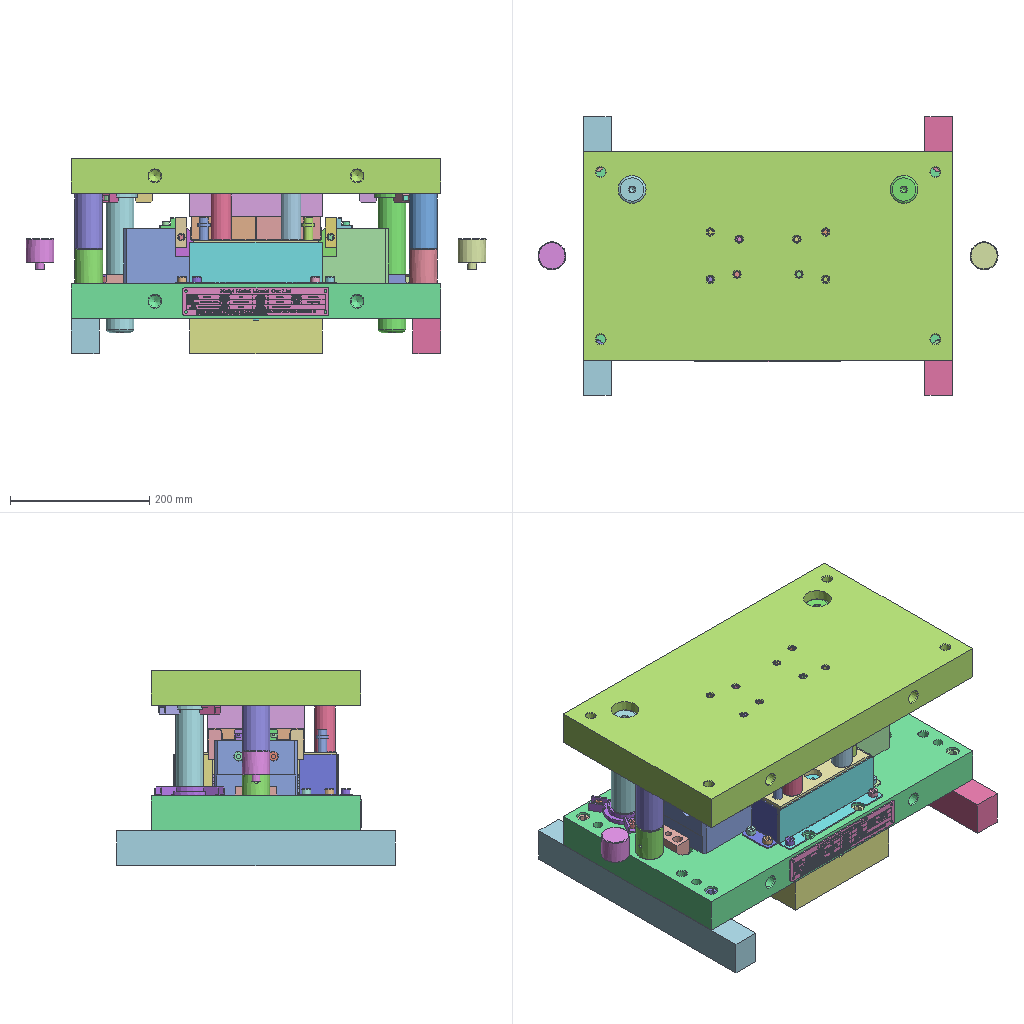Assembly | STEP file | 269 different items | 269 placed | box 660 x 400 x 280 mm
Parts list (item | name | quantity | parent item | size | volume):
1 | gslz 2016.10.28-6_id1002_x_t | x1 | in gslz 2016.10.28-6_x_t | 28.004 x 12 x 21.002 mm | 4222 mm3
2 | gslz 2016.10.28-6_id1006_x_t | x1 | in gslz 2016.10.28-6_x_t | 16 x 20 x 42.992 mm | 9660 mm3
3 | gslz 2016.10.28-6_id1010_x_t | x1 | in gslz 2016.10.28-6_x_t | 190 x 22 x 60 mm | 28864 mm3
4 | gslz 2016.10.28-6_id1014_x_t | x1 | in gslz 2016.10.28-6_x_t | - | 16189 mm3
5 | gslz 2016.10.28-6_id1018_x_t | x1 | in gslz 2016.10.28-6_x_t | 23 x 53 x 60 mm | 8271 mm3
6 | gslz 2016.10.28-6_id1022_x_t | x1 | in gslz 2016.10.28-6_x_t | 23 x 53 x 60 mm | 8271 mm3
7 | gslz 2016.10.28-6_id1026_x_t | x1 | in gslz 2016.10.28-6_x_t | 30 x 30 x 67.992 mm | 42323 mm3
8 | gslz 2016.10.28-6_id102_x_t | x1 | in gslz 2016.10.28-6_x_t | 18 x 18 x 67 mm | 8561 mm3
9 | gslz 2016.10.28-6_id1030_x_t | x1 | in gslz 2016.10.28-6_x_t | 30 x 30 x 67.992 mm | 42323 mm3
10 | gslz 2016.10.28-6_id1034_x_t | x1 | in gslz 2016.10.28-6_x_t | 25 x 110 x 40 mm | 96354 mm3
11 | gslz 2016.10.28-6_id1038_x_t | x1 | in gslz 2016.10.28-6_x_t | 190 x 300 x 50 mm | 2589810 mm3
12 | gslz 2016.10.28-6_id1042_x_t | x1 | in gslz 2016.10.28-6_x_t | 30 x 30 x 67.992 mm | 42323 mm3
13 | gslz 2016.10.28-6_id1046_x_t | x1 | in gslz 2016.10.28-6_x_t | 30 x 30 x 67.992 mm | 42323 mm3
14 | gslz 2016.10.28-6_id1050_x_t | x1 | in gslz 2016.10.28-6_x_t | 9.497 x 9.497 x 27.381 mm | 1219 mm3
15 | gslz 2016.10.28-6_id1054_x_t | x1 | in gslz 2016.10.28-6_x_t | 9.497 x 9.497 x 27.383 mm | 1219 mm3
16 | gslz 2016.10.28-6_id1058_x_t | x1 | in gslz 2016.10.28-6_x_t | 9.497 x 9.497 x 27.391 mm | 1219 mm3
17 | gslz 2016.10.28-6_id1062_x_t | x1 | in gslz 2016.10.28-6_x_t | 30 x 30 x 30 mm | 18212 mm3
18 | gslz 2016.10.28-6_id1066_x_t | x1 | in gslz 2016.10.28-6_x_t | 9.497 x 9.497 x 27.391 mm | 1219 mm3
19 | gslz 2016.10.28-6_id106_x_t | x1 | in gslz 2016.10.28-6_x_t | 18 x 18 x 67 mm | 8561 mm3
20 | gslz 2016.10.28-6_id1070_x_t | x1 | in gslz 2016.10.28-6_x_t | 530 x 300 x 50 mm | 7668211 mm3
21 | gslz 2016.10.28-6_id1074_x_t | x1 | in gslz 2016.10.28-6_x_t | 100 x 120 x 79 mm | 734438 mm3
22 | gslz 2016.10.28-6_id1078_x_t | x1 | in gslz 2016.10.28-6_x_t | 92 x 138 x 33.5 mm | 325352 mm3
23 | gslz 2016.10.28-6_id10_x_t | x1 | in gslz 2016.10.28-6_x_t | 25 x 60 x 25 mm | 30776 mm3
24 | gslz 2016.10.28-6_id110_x_t | x1 | in gslz 2016.10.28-6_x_t | 18 x 18 x 67 mm | 8561 mm3
25 | gslz 2016.10.28-6_id114_x_t | x1 | in gslz 2016.10.28-6_x_t | 18 x 18 x 67 mm | 8561 mm3
26 | gslz 2016.10.28-6_id118_x_t | x1 | in gslz 2016.10.28-6_x_t | 18 x 18 x 67 mm | 8561 mm3
27 | gslz 2016.10.28-6_id122_x_t | x1 | in gslz 2016.10.28-6_x_t | 13 x 13 x 23 mm | 1651 mm3
28 | gslz 2016.10.28-6_id126_x_t | x1 | in gslz 2016.10.28-6_x_t | 13 x 13 x 23 mm | 1651 mm3
29 | gslz 2016.10.28-6_id130_x_t | x1 | in gslz 2016.10.28-6_x_t | 13 x 13 x 23 mm | 1651 mm3
30 | gslz 2016.10.28-6_id134_x_t | x1 | in gslz 2016.10.28-6_x_t | 13 x 13 x 23 mm | 1651 mm3
31 | gslz 2016.10.28-6_id138_x_t | x1 | in gslz 2016.10.28-6_x_t | 13 x 13 x 23 mm | 1651 mm3
32 | gslz 2016.10.28-6_id142_x_t | x1 | in gslz 2016.10.28-6_x_t | 13 x 13 x 23 mm | 1651 mm3
33 | gslz 2016.10.28-6_id146_x_t | x1 | in gslz 2016.10.28-6_x_t | 13 x 13 x 23 mm | 1651 mm3
34 | gslz 2016.10.28-6_id14_x_t | x1 | in gslz 2016.10.28-6_x_t | 530 x 300 x 50 mm | 6912423 mm3
35 | gslz 2016.10.28-6_id150_x_t | x1 | in gslz 2016.10.28-6_x_t | 13 x 13 x 23 mm | 1651 mm3
36 | gslz 2016.10.28-6_id154_x_t | x1 | in gslz 2016.10.28-6_x_t | 13 x 13 x 23 mm | 1651 mm3
37 | gslz 2016.10.28-6_id158_x_t | x1 | in gslz 2016.10.28-6_x_t | 13 x 13 x 23 mm | 1651 mm3
38 | gslz 2016.10.28-6_id162_x_t | x1 | in gslz 2016.10.28-6_x_t | 13 x 13 x 23 mm | 1651 mm3
39 | gslz 2016.10.28-6_id166_x_t | x1 | in gslz 2016.10.28-6_x_t | 13 x 13 x 23 mm | 1651 mm3
40 | gslz 2016.10.28-6_id170_x_t | x1 | in gslz 2016.10.28-6_x_t | 40 x 40 x 50 mm | 56993 mm3
41 | gslz 2016.10.28-6_id174_x_t | x1 | in gslz 2016.10.28-6_x_t | 40 x 40 x 80 mm | 91705 mm3
42 | gslz 2016.10.28-6_id178_x_t | x1 | in gslz 2016.10.28-6_x_t | 13 x 13 x 52 mm | 3108 mm3
43 | gslz 2016.10.28-6_id182_x_t | x1 | in gslz 2016.10.28-6_x_t | 13 x 13 x 82 mm | 4616 mm3
44 | gslz 2016.10.28-6_id186_x_t | x1 | in gslz 2016.10.28-6_x_t | 40 x 40 x 45 mm | 44861 mm3
45 | gslz 2016.10.28-6_id18_x_t | x1 | in gslz 2016.10.28-6_x_t | 20 x 40 x 20 mm | 14270 mm3
46 | gslz 2016.10.28-6_id190_x_t | x1 | in gslz 2016.10.28-6_x_t | 40 x 40 x 45 mm | 44861 mm3
47 | gslz 2016.10.28-6_id194_x_t | x1 | in gslz 2016.10.28-6_x_t | 40 x 40 x 80 mm | 91705 mm3
48 | gslz 2016.10.28-6_id198_x_t | x1 | in gslz 2016.10.28-6_x_t | 40 x 40 x 50 mm | 56993 mm3
49 | gslz 2016.10.28-6_id202_x_t | x1 | in gslz 2016.10.28-6_x_t | 13 x 13 x 52 mm | 3108 mm3
50 | gslz 2016.10.28-6_id206_x_t | x1 | in gslz 2016.10.28-6_x_t | 13 x 13 x 82 mm | 4616 mm3
51 | gslz 2016.10.28-6_id210_x_t | x1 | in gslz 2016.10.28-6_x_t | 13 x 13 x 77 mm | 4365 mm3
52 | gslz 2016.10.28-6_id214_x_t | x1 | in gslz 2016.10.28-6_x_t | 13 x 13 x 77 mm | 4365 mm3
53 | gslz 2016.10.28-6_id218_x_t | x1 | in gslz 2016.10.28-6_x_t | 13 x 13 x 77 mm | 4365 mm3
54 | gslz 2016.10.28-6_id222_x_t | x1 | in gslz 2016.10.28-6_x_t | 13 x 13 x 77 mm | 4365 mm3
55 | gslz 2016.10.28-6_id226_x_t | x1 | in gslz 2016.10.28-6_x_t | 13 x 13 x 48 mm | 2907 mm3
56 | gslz 2016.10.28-6_id22_x_t | x1 | in gslz 2016.10.28-6_x_t | 180 x 230 x 32 mm | 1103435 mm3
57 | gslz 2016.10.28-6_id230_x_t | x1 | in gslz 2016.10.28-6_x_t | 13 x 13 x 48 mm | 2907 mm3
58 | gslz 2016.10.28-6_id234_x_t | x1 | in gslz 2016.10.28-6_x_t | 10 x 10 x 27 mm | 972.376 mm3
59 | gslz 2016.10.28-6_id238_x_t | x1 | in gslz 2016.10.28-6_x_t | 40 x 16 x 16 mm | 8856 mm3
60 | gslz 2016.10.28-6_id242_x_t | x1 | in gslz 2016.10.28-6_x_t | 10 x 10 x 27 mm | 972.376 mm3
61 | gslz 2016.10.28-6_id246_x_t | x1 | in gslz 2016.10.28-6_x_t | 16 x 40 x 16 mm | 8856 mm3
62 | gslz 2016.10.28-6_id250_x_t | x1 | in gslz 2016.10.28-6_x_t | 10 x 10 x 27 mm | 972.376 mm3
63 | gslz 2016.10.28-6_id254_x_t | x1 | in gslz 2016.10.28-6_x_t | 16 x 40 x 16 mm | 8856 mm3
64 | gslz 2016.10.28-6_id258_x_t | x1 | in gslz 2016.10.28-6_x_t | 10 x 10 x 26 mm | 944.102 mm3
65 | gslz 2016.10.28-6_id262_x_t | x1 | in gslz 2016.10.28-6_x_t | 30 x 16 x 16 mm | 6296 mm3
66 | gslz 2016.10.28-6_id266_x_t | x1 | in gslz 2016.10.28-6_x_t | 10 x 10 x 27 mm | 972.376 mm3
67 | gslz 2016.10.28-6_id26_x_t | x1 | in gslz 2016.10.28-6_x_t | 43 x 62 x 89 mm | 180403 mm3
68 | gslz 2016.10.28-6_id270_x_t | x1 | in gslz 2016.10.28-6_x_t | 16 x 40 x 16 mm | 8856 mm3
69 | gslz 2016.10.28-6_id274_x_t | x1 | in gslz 2016.10.28-6_x_t | 10 x 10 x 27 mm | 972.376 mm3
70 | gslz 2016.10.28-6_id278_x_t | x1 | in gslz 2016.10.28-6_x_t | 16 x 40 x 16 mm | 8856 mm3
71 | gslz 2016.10.28-6_id282_x_t | x1 | in gslz 2016.10.28-6_x_t | 10 x 10 x 26 mm | 944.102 mm3
72 | gslz 2016.10.28-6_id286_x_t | x1 | in gslz 2016.10.28-6_x_t | 30 x 16 x 16 mm | 6296 mm3
73 | gslz 2016.10.28-6_id290_x_t | x1 | in gslz 2016.10.28-6_x_t | 16 x 16 x 85 mm | 7560 mm3
74 | gslz 2016.10.28-6_id294_x_t | x1 | in gslz 2016.10.28-6_x_t | 16 x 16 x 85 mm | 7560 mm3
75 | gslz 2016.10.28-6_id298_x_t | x1 | in gslz 2016.10.28-6_x_t | 16 x 16 x 85 mm | 7560 mm3
76 | gslz 2016.10.28-6_id302_x_t | x1 | in gslz 2016.10.28-6_x_t | 16 x 16 x 85 mm | 7560 mm3
77 | gslz 2016.10.28-6_id306_x_t | x1 | in gslz 2016.10.28-6_x_t | 16 x 16 x 85 mm | 7560 mm3
78 | gslz 2016.10.28-6_id30_x_t | x1 | in gslz 2016.10.28-6_x_t | 43 x 62 x 89 mm | 180403 mm3
79 | gslz 2016.10.28-6_id310_x_t | x1 | in gslz 2016.10.28-6_x_t | 16 x 16 x 85 mm | 7560 mm3
80 | gslz 2016.10.28-6_id314_x_t | x1 | in gslz 2016.10.28-6_x_t | 16 x 16 x 85 mm | 7560 mm3
81 | gslz 2016.10.28-6_id318_x_t | x1 | in gslz 2016.10.28-6_x_t | 16 x 16 x 85 mm | 7560 mm3
82 | gslz 2016.10.28-6_id322_x_t | x1 | in gslz 2016.10.28-6_x_t | 190 x 138 x 33 mm | 763181 mm3
83 | gslz 2016.10.28-6_id326_x_t | x1 | in gslz 2016.10.28-6_x_t | 12 x 12 x 12 mm | 1092 mm3
84 | gslz 2016.10.28-6_id330_x_t | x1 | in gslz 2016.10.28-6_x_t | 9.997 x 9.994 x 45 mm | 331.132 mm3
85 | gslz 2016.10.28-6_id334_x_t | x1 | in gslz 2016.10.28-6_x_t | 10 x 10 x 48 mm | 2492 mm3
86 | gslz 2016.10.28-6_id338_x_t | x1 | in gslz 2016.10.28-6_x_t | 9.997 x 9.994 x 45 mm | 331.132 mm3
87 | gslz 2016.10.28-6_id342_x_t | x1 | in gslz 2016.10.28-6_x_t | 12 x 12 x 12 mm | 1092 mm3
88 | gslz 2016.10.28-6_id346_x_t | x1 | in gslz 2016.10.28-6_x_t | 10 x 10 x 48 mm | 2492 mm3
89 | gslz 2016.10.28-6_id34_x_t | x1 | in gslz 2016.10.28-6_x_t | 43 x 62 x 89 mm | 180411 mm3
90 | gslz 2016.10.28-6_id350_x_t | x1 | in gslz 2016.10.28-6_x_t | 9.997 x 9.994 x 45 mm | 331.132 mm3
91 | gslz 2016.10.28-6_id354_x_t | x1 | in gslz 2016.10.28-6_x_t | 12 x 12 x 12 mm | 1092 mm3
92 | gslz 2016.10.28-6_id358_x_t | x1 | in gslz 2016.10.28-6_x_t | 10 x 10 x 48 mm | 2492 mm3
93 | gslz 2016.10.28-6_id362_x_t | x1 | in gslz 2016.10.28-6_x_t | 9.997 x 9.994 x 45 mm | 331.132 mm3
94 | gslz 2016.10.28-6_id366_x_t | x1 | in gslz 2016.10.28-6_x_t | 12 x 12 x 12 mm | 1092 mm3
95 | gslz 2016.10.28-6_id370_x_t | x1 | in gslz 2016.10.28-6_x_t | 10 x 10 x 48 mm | 2492 mm3
96 | gslz 2016.10.28-6_id374_x_t | x1 | in gslz 2016.10.28-6_x_t | 9.997 x 9.994 x 45 mm | 330.149 mm3
97 | gslz 2016.10.28-6_id378_x_t | x1 | in gslz 2016.10.28-6_x_t | 12 x 12 x 12 mm | 1092 mm3
98 | gslz 2016.10.28-6_id382_x_t | x1 | in gslz 2016.10.28-6_x_t | 10 x 10 x 48 mm | 2492 mm3
99 | gslz 2016.10.28-6_id386_x_t | x1 | in gslz 2016.10.28-6_x_t | 9.997 x 9.994 x 45 mm | 330.149 mm3
100 | gslz 2016.10.28-6_id38_x_t | x1 | in gslz 2016.10.28-6_x_t | 82.449 x 96 x 19.004 mm | 9470 mm3
101 | gslz 2016.10.28-6_id390_x_t | x1 | in gslz 2016.10.28-6_x_t | 12 x 12 x 12 mm | 1092 mm3
102 | gslz 2016.10.28-6_id394_x_t | x1 | in gslz 2016.10.28-6_x_t | 10 x 10 x 48 mm | 2492 mm3
103 | gslz 2016.10.28-6_id398_x_t | x1 | in gslz 2016.10.28-6_x_t | 12 x 12 x 12 mm | 1092 mm3
104 | gslz 2016.10.28-6_id402_x_t | x1 | in gslz 2016.10.28-6_x_t | 9.997 x 9.994 x 45 mm | 330.149 mm3
105 | gslz 2016.10.28-6_id406_x_t | x1 | in gslz 2016.10.28-6_x_t | 10 x 10 x 48 mm | 2492 mm3
106 | gslz 2016.10.28-6_id410_x_t | x1 | in gslz 2016.10.28-6_x_t | 12 x 12 x 12 mm | 1092 mm3
107 | gslz 2016.10.28-6_id414_x_t | x1 | in gslz 2016.10.28-6_x_t | 10 x 10 x 48 mm | 2492 mm3
108 | gslz 2016.10.28-6_id418_x_t | x1 | in gslz 2016.10.28-6_x_t | 9.997 x 9.994 x 45 mm | 330.149 mm3
109 | gslz 2016.10.28-6_id422_x_t | x1 | in gslz 2016.10.28-6_x_t | 10 x 10 x 26 mm | 944.102 mm3
110 | gslz 2016.10.28-6_id426_x_t | x1 | in gslz 2016.10.28-6_x_t | 10 x 10 x 26 mm | 944.102 mm3
111 | gslz 2016.10.28-6_id42_x_t | x1 | in gslz 2016.10.28-6_x_t | 92 x 138 x 33.5 mm | 323745 mm3
112 | gslz 2016.10.28-6_id430_x_t | x1 | in gslz 2016.10.28-6_x_t | 10 x 10 x 26 mm | 944.102 mm3
113 | gslz 2016.10.28-6_id434_x_t | x1 | in gslz 2016.10.28-6_x_t | 56.6 x 32.6 x 114 mm | 58332 mm3
114 | gslz 2016.10.28-6_id438_x_t | x1 | in gslz 2016.10.28-6_x_t | 10 x 10 x 26 mm | 944.102 mm3
115 | gslz 2016.10.28-6_id442_x_t | x1 | in gslz 2016.10.28-6_x_t | 64 x 40 x 40 mm | 16525 mm3
116 | gslz 2016.10.28-6_id446_x_t | x1 | in gslz 2016.10.28-6_x_t | 10 x 10 x 26 mm | 944.102 mm3
117 | gslz 2016.10.28-6_id450_x_t | x1 | in gslz 2016.10.28-6_x_t | 64 x 40 x 40 mm | 16525 mm3
118 | gslz 2016.10.28-6_id454_x_t | x1 | in gslz 2016.10.28-6_x_t | 10 x 10 x 26 mm | 944.102 mm3
119 | gslz 2016.10.28-6_id458_x_t | x1 | in gslz 2016.10.28-6_x_t | 10 x 10 x 26 mm | 944.102 mm3
120 | gslz 2016.10.28-6_id462_x_t | x1 | in gslz 2016.10.28-6_x_t | 10 x 10 x 26 mm | 944.102 mm3
121 | gslz 2016.10.28-6_id466_x_t | x1 | in gslz 2016.10.28-6_x_t | 56.6 x 32.6 x 114 mm | 58331 mm3
122 | gslz 2016.10.28-6_id46_x_t | x1 | in gslz 2016.10.28-6_x_t | 82.449 x 96 x 19.004 mm | 9463 mm3
123 | gslz 2016.10.28-6_id470_x_t | x1 | in gslz 2016.10.28-6_x_t | 12 x 12 x 12 mm | 1092 mm3
124 | gslz 2016.10.28-6_id474_x_t | x1 | in gslz 2016.10.28-6_x_t | 12 x 12 x 12 mm | 1092 mm3
125 | gslz 2016.10.28-6_id478_x_t | x1 | in gslz 2016.10.28-6_x_t | 12 x 12 x 12 mm | 1092 mm3
126 | gslz 2016.10.28-6_id482_x_t | x1 | in gslz 2016.10.28-6_x_t | 12 x 12 x 12 mm | 1092 mm3
127 | gslz 2016.10.28-6_id486_x_t | x1 | in gslz 2016.10.28-6_x_t | 18 x 18 x 110 mm | 13813 mm3
128 | gslz 2016.10.28-6_id490_x_t | x1 | in gslz 2016.10.28-6_x_t | 18 x 18 x 110 mm | 13813 mm3
129 | gslz 2016.10.28-6_id494_x_t | x1 | in gslz 2016.10.28-6_x_t | 18 x 18 x 110 mm | 13813 mm3
130 | gslz 2016.10.28-6_id498_x_t | x1 | in gslz 2016.10.28-6_x_t | 18 x 18 x 110 mm | 13813 mm3
131 | gslz 2016.10.28-6_id502_x_t | x1 | in gslz 2016.10.28-6_x_t | 6 x 6 x 13 mm | 209.85 mm3
132 | gslz 2016.10.28-6_id506_x_t | x1 | in gslz 2016.10.28-6_x_t | 8 x 8 x 8 mm | 323.66 mm3
133 | gslz 2016.10.28-6_id50_x_t | x1 | in gslz 2016.10.28-6_x_t | 40.005 x 40.005 x 103 mm | 60665 mm3
134 | gslz 2016.10.28-6_id510_x_t | x1 | in gslz 2016.10.28-6_x_t | 5.996 x 5.994 x 11 mm | 66.438 mm3
135 | gslz 2016.10.28-6_id514_x_t | x1 | in gslz 2016.10.28-6_x_t | 6 x 6 x 13 mm | 209.85 mm3
136 | gslz 2016.10.28-6_id518_x_t | x1 | in gslz 2016.10.28-6_x_t | 8 x 8 x 8 mm | 323.66 mm3
137 | gslz 2016.10.28-6_id522_x_t | x1 | in gslz 2016.10.28-6_x_t | 5.996 x 5.994 x 11 mm | 66.438 mm3
138 | gslz 2016.10.28-6_id526_x_t | x1 | in gslz 2016.10.28-6_x_t | 6 x 6 x 13 mm | 209.85 mm3
139 | gslz 2016.10.28-6_id530_x_t | x1 | in gslz 2016.10.28-6_x_t | 8 x 8 x 8 mm | 323.66 mm3
140 | gslz 2016.10.28-6_id534_x_t | x1 | in gslz 2016.10.28-6_x_t | 5.996 x 5.994 x 11 mm | 66.438 mm3
141 | gslz 2016.10.28-6_id538_x_t | x1 | in gslz 2016.10.28-6_x_t | 6 x 6 x 13 mm | 209.85 mm3
142 | gslz 2016.10.28-6_id542_x_t | x1 | in gslz 2016.10.28-6_x_t | 8 x 8 x 8 mm | 323.66 mm3
143 | gslz 2016.10.28-6_id546_x_t | x1 | in gslz 2016.10.28-6_x_t | 5.996 x 5.994 x 11 mm | 66.438 mm3
144 | gslz 2016.10.28-6_id54_x_t | x1 | in gslz 2016.10.28-6_x_t | 40.005 x 40.005 x 103 mm | 60665 mm3
145 | gslz 2016.10.28-6_id550_x_t | x1 | in gslz 2016.10.28-6_x_t | 6 x 6 x 13 mm | 209.85 mm3
146 | gslz 2016.10.28-6_id554_x_t | x1 | in gslz 2016.10.28-6_x_t | 8 x 8 x 8 mm | 323.66 mm3
147 | gslz 2016.10.28-6_id558_x_t | x1 | in gslz 2016.10.28-6_x_t | 5.996 x 5.994 x 11 mm | 66.438 mm3
148 | gslz 2016.10.28-6_id562_x_t | x1 | in gslz 2016.10.28-6_x_t | 6 x 6 x 13 mm | 209.85 mm3
149 | gslz 2016.10.28-6_id566_x_t | x1 | in gslz 2016.10.28-6_x_t | 8 x 8 x 8 mm | 323.66 mm3
150 | gslz 2016.10.28-6_id570_x_t | x1 | in gslz 2016.10.28-6_x_t | 5.996 x 5.994 x 11 mm | 66.438 mm3
151 | gslz 2016.10.28-6_id574_x_t | x1 | in gslz 2016.10.28-6_x_t | 6 x 6 x 13 mm | 209.85 mm3
152 | gslz 2016.10.28-6_id578_x_t | x1 | in gslz 2016.10.28-6_x_t | 8 x 8 x 8 mm | 323.66 mm3
153 | gslz 2016.10.28-6_id582_x_t | x1 | in gslz 2016.10.28-6_x_t | 5.996 x 5.994 x 11 mm | 66.438 mm3
154 | gslz 2016.10.28-6_id586_x_t | x1 | in gslz 2016.10.28-6_x_t | 6 x 6 x 13 mm | 209.85 mm3
155 | gslz 2016.10.28-6_id58_x_t | x1 | in gslz 2016.10.28-6_x_t | 40.005 x 40.005 x 103 mm | 60664 mm3
156 | gslz 2016.10.28-6_id590_x_t | x1 | in gslz 2016.10.28-6_x_t | 8 x 8 x 8 mm | 323.66 mm3
157 | gslz 2016.10.28-6_id594_x_t | x1 | in gslz 2016.10.28-6_x_t | 5.996 x 5.994 x 11 mm | 66.438 mm3
158 | gslz 2016.10.28-6_id598_x_t | x1 | in gslz 2016.10.28-6_x_t | 6 x 6 x 13 mm | 209.85 mm3
159 | gslz 2016.10.28-6_id602_x_t | x1 | in gslz 2016.10.28-6_x_t | 8 x 8 x 8 mm | 323.66 mm3
160 | gslz 2016.10.28-6_id606_x_t | x1 | in gslz 2016.10.28-6_x_t | 5.996 x 5.994 x 11 mm | 66.438 mm3
161 | gslz 2016.10.28-6_id610_x_t | x1 | in gslz 2016.10.28-6_x_t | 6 x 6 x 13 mm | 209.85 mm3
162 | gslz 2016.10.28-6_id614_x_t | x1 | in gslz 2016.10.28-6_x_t | 8 x 8 x 8 mm | 323.66 mm3
163 | gslz 2016.10.28-6_id618_x_t | x1 | in gslz 2016.10.28-6_x_t | 5.996 x 5.994 x 11 mm | 66.438 mm3
164 | gslz 2016.10.28-6_id622_x_t | x1 | in gslz 2016.10.28-6_x_t | 6 x 6 x 13 mm | 209.85 mm3
165 | gslz 2016.10.28-6_id626_x_t | x1 | in gslz 2016.10.28-6_x_t | 8 x 8 x 8 mm | 323.66 mm3
166 | gslz 2016.10.28-6_id62_x_t | x1 | in gslz 2016.10.28-6_x_t | 40.005 x 40.005 x 103 mm | 60665 mm3
167 | gslz 2016.10.28-6_id630_x_t | x1 | in gslz 2016.10.28-6_x_t | 5.996 x 5.994 x 11 mm | 66.438 mm3
168 | gslz 2016.10.28-6_id634_x_t | x1 | in gslz 2016.10.28-6_x_t | 5.996 x 5.994 x 11 mm | 66.438 mm3
169 | gslz 2016.10.28-6_id638_x_t | x1 | in gslz 2016.10.28-6_x_t | 8 x 8 x 8 mm | 323.66 mm3
170 | gslz 2016.10.28-6_id642_x_t | x1 | in gslz 2016.10.28-6_x_t | 6 x 6 x 13 mm | 209.85 mm3
171 | gslz 2016.10.28-6_id646_x_t | x1 | in gslz 2016.10.28-6_x_t | 10 x 10 x 27 mm | 972.376 mm3
172 | gslz 2016.10.28-6_id650_x_t | x1 | in gslz 2016.10.28-6_x_t | 10 x 10 x 27 mm | 972.376 mm3
173 | gslz 2016.10.28-6_id654_x_t | x1 | in gslz 2016.10.28-6_x_t | 10 x 10 x 27 mm | 972.376 mm3
174 | gslz 2016.10.28-6_id658_x_t | x1 | in gslz 2016.10.28-6_x_t | 10 x 10 x 27 mm | 972.376 mm3
175 | gslz 2016.10.28-6_id662_x_t | x1 | in gslz 2016.10.28-6_x_t | 10 x 10 x 27 mm | 972.376 mm3
176 | gslz 2016.10.28-6_id666_x_t | x1 | in gslz 2016.10.28-6_x_t | 10 x 10 x 27 mm | 972.376 mm3
177 | gslz 2016.10.28-6_id66_x_t | x1 | in gslz 2016.10.28-6_x_t | 40.005 x 40.005 x 103 mm | 60665 mm3
178 | gslz 2016.10.28-6_id670_x_t | x1 | in gslz 2016.10.28-6_x_t | 20 x 40 x 20 mm | 14272 mm3
179 | gslz 2016.10.28-6_id674_x_t | x1 | in gslz 2016.10.28-6_x_t | 10 x 10 x 27 mm | 972.376 mm3
180 | gslz 2016.10.28-6_id678_x_t | x1 | in gslz 2016.10.28-6_x_t | 10 x 10 x 27 mm | 972.376 mm3
181 | gslz 2016.10.28-6_id682_x_t | x1 | in gslz 2016.10.28-6_x_t | 28.004 x 12 x 21.002 mm | 4222 mm3
182 | gslz 2016.10.28-6_id686_x_t | x1 | in gslz 2016.10.28-6_x_t | 10 x 10 x 21 mm | 802.73 mm3
183 | gslz 2016.10.28-6_id690_x_t | x1 | in gslz 2016.10.28-6_x_t | 16 x 16 x 92 mm | 8110 mm3
184 | gslz 2016.10.28-6_id694_x_t | x1 | in gslz 2016.10.28-6_x_t | 100 x 120 x 79 mm | 734438 mm3
185 | gslz 2016.10.28-6_id698_x_t | x1 | in gslz 2016.10.28-6_x_t | 20 x 16 x 12 mm | 2982 mm3
186 | gslz 2016.10.28-6_id6_x_t | x1 | in gslz 2016.10.28-6_x_t | 25 x 60 x 25 mm | 30776 mm3
187 | gslz 2016.10.28-6_id702_x_t | x1 | in gslz 2016.10.28-6_x_t | 16 x 20 x 42.992 mm | 9660 mm3
188 | gslz 2016.10.28-6_id706_x_t | x1 | in gslz 2016.10.28-6_x_t | 10 x 10 x 27 mm | 972.376 mm3
189 | gslz 2016.10.28-6_id70_x_t | x1 | in gslz 2016.10.28-6_x_t | 40.005 x 40.005 x 103 mm | 60665 mm3
190 | gslz 2016.10.28-6_id710_x_t | x1 | in gslz 2016.10.28-6_x_t | 10 x 22 x 10 mm | 831.004 mm3
191 | gslz 2016.10.28-6_id714_x_t | x1 | in gslz 2016.10.28-6_x_t | 16 x 16 x 92 mm | 8110 mm3
192 | gslz 2016.10.28-6_id718_x_t | x1 | in gslz 2016.10.28-6_x_t | 10 x 10 x 26 mm | 944.102 mm3
193 | gslz 2016.10.28-6_id722_x_t | x1 | in gslz 2016.10.28-6_x_t | 82 x 13 x 13 mm | 4616 mm3
194 | gslz 2016.10.28-6_id726_x_t | x1 | in gslz 2016.10.28-6_x_t | 10 x 22 x 10 mm | 831.004 mm3
195 | gslz 2016.10.28-6_id730_x_t | x1 | in gslz 2016.10.28-6_x_t | 82 x 13 x 13 mm | 4616 mm3
196 | gslz 2016.10.28-6_id734_x_t | x1 | in gslz 2016.10.28-6_x_t | 16 x 20 x 42.992 mm | 9660 mm3
197 | gslz 2016.10.28-6_id738_x_t | x1 | in gslz 2016.10.28-6_x_t | 28.003 x 12 x 21.002 mm | 4221 mm3
198 | gslz 2016.10.28-6_id742_x_t | x1 | in gslz 2016.10.28-6_x_t | 16 x 16 x 92 mm | 8110 mm3
199 | gslz 2016.10.28-6_id746_x_t | x1 | in gslz 2016.10.28-6_x_t | 25 x 110 x 40 mm | 96354 mm3
200 | gslz 2016.10.28-6_id74_x_t | x1 | in gslz 2016.10.28-6_x_t | 12 x 12 x 66 mm | 6932 mm3
201 | gslz 2016.10.28-6_id750_x_t | x1 | in gslz 2016.10.28-6_x_t | 16 x 16 x 92 mm | 8110 mm3
202 | gslz 2016.10.28-6_id754_x_t | x1 | in gslz 2016.10.28-6_x_t | 30 x 16 x 16 mm | 6296 mm3
203 | gslz 2016.10.28-6_id758_x_t | x1 | in gslz 2016.10.28-6_x_t | 10 x 10 x 27 mm | 972.376 mm3
204 | gslz 2016.10.28-6_id762_x_t | x1 | in gslz 2016.10.28-6_x_t | 10 x 10 x 26 mm | 944.102 mm3
205 | gslz 2016.10.28-6_id766_x_t | x1 | in gslz 2016.10.28-6_x_t | 30 x 16 x 16 mm | 6296 mm3
206 | gslz 2016.10.28-6_id770_x_t | x1 | in gslz 2016.10.28-6_x_t | 10 x 22 x 10 mm | 831.004 mm3
207 | gslz 2016.10.28-6_id774_x_t | x1 | in gslz 2016.10.28-6_x_t | 10 x 22 x 10 mm | 831.004 mm3
208 | gslz 2016.10.28-6_id778_x_t | x1 | in gslz 2016.10.28-6_x_t | 10 x 10 x 27 mm | 972.376 mm3
209 | gslz 2016.10.28-6_id782_x_t | x1 | in gslz 2016.10.28-6_x_t | 10 x 10 x 27 mm | 972.376 mm3
210 | gslz 2016.10.28-6_id786_x_t | x1 | in gslz 2016.10.28-6_x_t | 10 x 10 x 21 mm | 802.73 mm3
211 | gslz 2016.10.28-6_id78_x_t | x1 | in gslz 2016.10.28-6_x_t | 12 x 12 x 66 mm | 6932 mm3
212 | gslz 2016.10.28-6_id790_x_t | x1 | in gslz 2016.10.28-6_x_t | 16 x 16 x 92 mm | 8110 mm3
213 | gslz 2016.10.28-6_id794_x_t | x1 | in gslz 2016.10.28-6_x_t | 16 x 16 x 92 mm | 8110 mm3
214 | gslz 2016.10.28-6_id798_x_t | x1 | in gslz 2016.10.28-6_x_t | 16 x 16 x 92 mm | 8110 mm3
215 | gslz 2016.10.28-6_id802_x_t | x1 | in gslz 2016.10.28-6_x_t | 16 x 16 x 92 mm | 8110 mm3
216 | gslz 2016.10.28-6_id806_x_t | x1 | in gslz 2016.10.28-6_x_t | 82 x 13 x 13 mm | 4616 mm3
217 | gslz 2016.10.28-6_id810_x_t | x1 | in gslz 2016.10.28-6_x_t | 82 x 13 x 13 mm | 4616 mm3
218 | gslz 2016.10.28-6_id814_x_t | x1 | in gslz 2016.10.28-6_x_t | 24.6 x 18.9 x 13 mm | 2016 mm3
219 | gslz 2016.10.28-6_id818_x_t | x1 | in gslz 2016.10.28-6_x_t | 13 x 13 x 23 mm | 1651 mm3
220 | gslz 2016.10.28-6_id822_x_t | x1 | in gslz 2016.10.28-6_x_t | 13 x 13 x 23 mm | 1651 mm3
221 | gslz 2016.10.28-6_id826_x_t | x1 | in gslz 2016.10.28-6_x_t | 28.668 x 30.754 x 13 mm | 2016 mm3
222 | gslz 2016.10.28-6_id82_x_t | x1 | in gslz 2016.10.28-6_x_t | 12 x 12 x 66 mm | 6932 mm3
223 | gslz 2016.10.28-6_id830_x_t | x1 | in gslz 2016.10.28-6_x_t | 50.8 x 50.8 x 237 mm | 300382 mm3
224 | gslz 2016.10.28-6_id834_x_t | x1 | in gslz 2016.10.28-6_x_t | 28.668 x 30.754 x 13 mm | 2016 mm3
225 | gslz 2016.10.28-6_id838_x_t | x1 | in gslz 2016.10.28-6_x_t | 86.634 x 100.036 x 63 mm | 56971 mm3
226 | gslz 2016.10.28-6_id842_x_t | x1 | in gslz 2016.10.28-6_x_t | 13 x 13 x 23 mm | 1651 mm3
227 | gslz 2016.10.28-6_id846_x_t | x1 | in gslz 2016.10.28-6_x_t | 13 x 13 x 23 mm | 1651 mm3
228 | gslz 2016.10.28-6_id850_x_t | x1 | in gslz 2016.10.28-6_x_t | 13 x 13 x 23 mm | 1651 mm3
229 | gslz 2016.10.28-6_id854_x_t | x1 | in gslz 2016.10.28-6_x_t | 13 x 13 x 23 mm | 1651 mm3
230 | gslz 2016.10.28-6_id858_x_t | x1 | in gslz 2016.10.28-6_x_t | 13 x 13 x 23 mm | 1651 mm3
231 | gslz 2016.10.28-6_id862_x_t | x1 | in gslz 2016.10.28-6_x_t | 13 x 13 x 23 mm | 1651 mm3
232 | gslz 2016.10.28-6_id866_x_t | x1 | in gslz 2016.10.28-6_x_t | 86.634 x 100.036 x 63 mm | 56971 mm3
233 | gslz 2016.10.28-6_id86_x_t | x1 | in gslz 2016.10.28-6_x_t | 12 x 12 x 66 mm | 6932 mm3
234 | gslz 2016.10.28-6_id870_x_t | x1 | in gslz 2016.10.28-6_x_t | 24.6 x 18.9 x 13 mm | 2016 mm3
235 | gslz 2016.10.28-6_id874_x_t | x1 | in gslz 2016.10.28-6_x_t | 50.8 x 50.8 x 237 mm | 300382 mm3
236 | gslz 2016.10.28-6_id878_x_t | x1 | in gslz 2016.10.28-6_x_t | 28.668 x 30.754 x 13 mm | 2016 mm3
237 | gslz 2016.10.28-6_id882_x_t | x1 | in gslz 2016.10.28-6_x_t | 13 x 13 x 23 mm | 1651 mm3
238 | gslz 2016.10.28-6_id886_x_t | x1 | in gslz 2016.10.28-6_x_t | 28.668 x 30.754 x 13 mm | 2016 mm3
239 | gslz 2016.10.28-6_id890_x_t | x1 | in gslz 2016.10.28-6_x_t | 13 x 13 x 23 mm | 1651 mm3
240 | gslz 2016.10.28-6_id894_x_t | x1 | in gslz 2016.10.28-6_x_t | 13 x 13 x 23 mm | 1651 mm3
241 | gslz 2016.10.28-6_id898_x_t | x1 | in gslz 2016.10.28-6_x_t | 13 x 13 x 23 mm | 1651 mm3
242 | gslz 2016.10.28-6_id902_x_t | x1 | in gslz 2016.10.28-6_x_t | 16 x 16 x 102 mm | 8895 mm3
243 | gslz 2016.10.28-6_id906_x_t | x1 | in gslz 2016.10.28-6_x_t | 16 x 16 x 102 mm | 8895 mm3
244 | gslz 2016.10.28-6_id90_x_t | x1 | in gslz 2016.10.28-6_x_t | 18 x 18 x 67 mm | 8561 mm3
245 | gslz 2016.10.28-6_id910_x_t | x1 | in gslz 2016.10.28-6_x_t | 13 x 13 x 42 mm | 2606 mm3
246 | gslz 2016.10.28-6_id914_x_t | x1 | in gslz 2016.10.28-6_x_t | 30 x 30 x 30 mm | 18212 mm3
247 | gslz 2016.10.28-6_id918_x_t | x1 | in gslz 2016.10.28-6_x_t | 13 x 13 x 42 mm | 2606 mm3
248 | gslz 2016.10.28-6_id922_x_t | x1 | in gslz 2016.10.28-6_x_t | 30 x 30 x 30 mm | 18212 mm3
249 | gslz 2016.10.28-6_id926_x_t | x1 | in gslz 2016.10.28-6_x_t | 13 x 13 x 42 mm | 2606 mm3
250 | gslz 2016.10.28-6_id930_x_t | x1 | in gslz 2016.10.28-6_x_t | 30 x 30 x 30 mm | 18212 mm3
251 | gslz 2016.10.28-6_id934_x_t | x1 | in gslz 2016.10.28-6_x_t | 13 x 13 x 42 mm | 2606 mm3
252 | gslz 2016.10.28-6_id938_x_t | x1 | in gslz 2016.10.28-6_x_t | 30 x 30 x 30 mm | 18212 mm3
253 | gslz 2016.10.28-6_id942_x_t | x1 | in gslz 2016.10.28-6_x_t | 13 x 13 x 42 mm | 2606 mm3
254 | gslz 2016.10.28-6_id946_x_t | x1 | in gslz 2016.10.28-6_x_t | 190 x 22 x 60 mm | 28864 mm3
255 | gslz 2016.10.28-6_id94_x_t | x1 | in gslz 2016.10.28-6_x_t | 18 x 18 x 67 mm | 8561 mm3
256 | gslz 2016.10.28-6_id950_x_t | x1 | in gslz 2016.10.28-6_x_t | 23 x 53 x 60 mm | 8271 mm3
257 | gslz 2016.10.28-6_id954_x_t | x1 | in gslz 2016.10.28-6_x_t | 23 x 53 x 60 mm | 8271 mm3
258 | gslz 2016.10.28-6_id958_x_t | x1 | in gslz 2016.10.28-6_x_t | 40 x 400 x 50 mm | 781861 mm3
259 | gslz 2016.10.28-6_id962_x_t | x1 | in gslz 2016.10.28-6_x_t | 40 x 400 x 50 mm | 781861 mm3
260 | gslz 2016.10.28-6_id966_x_t | x1 | in gslz 2016.10.28-6_x_t | 19.21 x 29.71 x 21.004 mm | 4221 mm3
261 | gslz 2016.10.28-6_id970_x_t | x1 | in gslz 2016.10.28-6_x_t | 18.394 x 29.644 x 21.004 mm | 4221 mm3
262 | gslz 2016.10.28-6_id974_x_t | x1 | in gslz 2016.10.28-6_x_t | 29.124 x 15.503 x 21.011 mm | 4221 mm3
263 | gslz 2016.10.28-6_id978_x_t | x1 | in gslz 2016.10.28-6_x_t | 19.21 x 29.71 x 21.004 mm | 4221 mm3
264 | gslz 2016.10.28-6_id982_x_t | x1 | in gslz 2016.10.28-6_x_t | 29.101 x 15.421 x 21.004 mm | 4221 mm3
265 | gslz 2016.10.28-6_id986_x_t | x1 | in gslz 2016.10.28-6_x_t | 18.394 x 29.644 x 21.004 mm | 4221 mm3
266 | gslz 2016.10.28-6_id98_x_t | x1 | in gslz 2016.10.28-6_x_t | 18 x 18 x 67 mm | 8561 mm3
267 | gslz 2016.10.28-6_id990_x_t | x1 | in gslz 2016.10.28-6_x_t | 20 x 16 x 12 mm | 2982 mm3
268 | gslz 2016.10.28-6_id994_x_t | x1 | in gslz 2016.10.28-6_x_t | 16 x 20 x 42.992 mm | 9660 mm3
269 | gslz 2016.10.28-6_id998_x_t | x1 | in gslz 2016.10.28-6_x_t | 28.003 x 12 x 21.002 mm | 4221 mm3